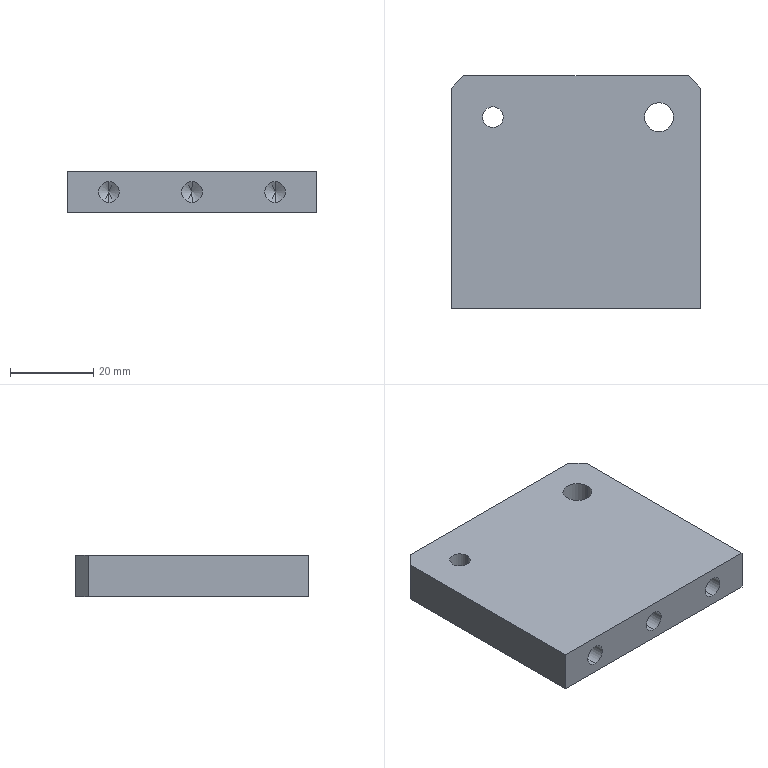Part | STEP file | PN_0082 transport limit mounting plate | 1 solid | 24 faces | box 60 x 56 x 10 mm | volume 31898 mm3 | cylinder 10 | plane 8 | cone 6 | commonest cylinder face diameters 5 x8 7 x2